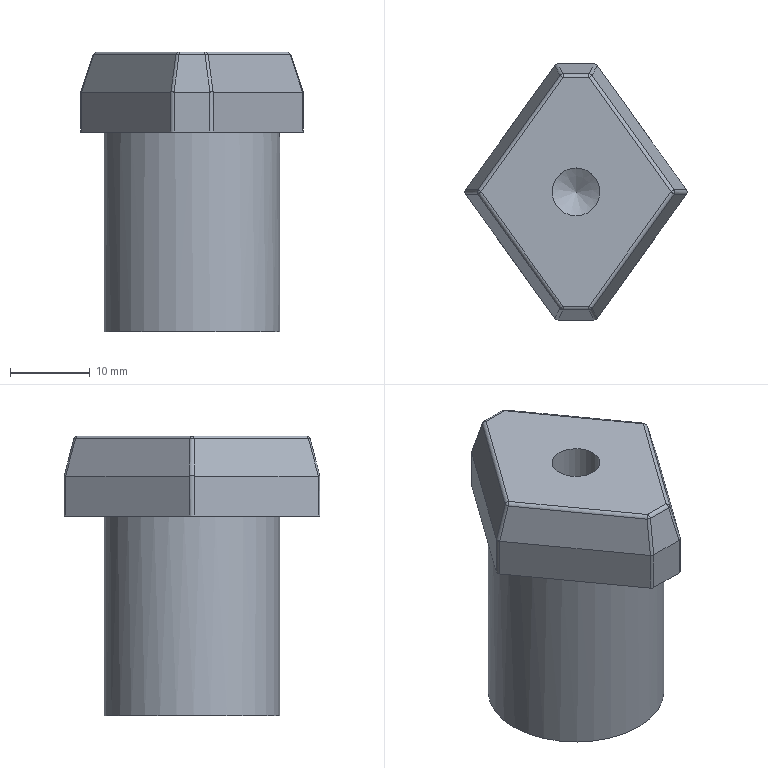Part | NX | features solid 2 | 1 solid | 45 faces | box 27.768 x 32 x 35 mm | volume 14194 mm3 | cylinder 20 | plane 18 | sphere 6 | cone 1 | commonest cylinder face diameters 1 x18 6 x1 22 x1
STEP:
#1=CARTESIAN_POINT('',(-816.022,-207.724,54.62));
#2=VERTEX_POINT('',#1);
#3=CARTESIAN_POINT('',(-816.022,-220.564,54.62));
#4=VERTEX_POINT('',#3);
#5=CARTESIAN_POINT('',(-807.09,-214.144,54.62));
#6=DIRECTION('',(0.,0.,1.));
#7=DIRECTION('',(1.,0.,0.));
#8=AXIS2_PLACEMENT_3D('',#5,#6,#7);
#9=CIRCLE('',#8,11.);
#10=EDGE_CURVE('',#2,#4,#9,.T.);
#11=ORIENTED_EDGE('',*,*,#10,.F.);
#12=CARTESIAN_POINT('',(-798.158,-207.724,54.62));
#13=VERTEX_POINT('',#12);
#14=CARTESIAN_POINT('',(-807.09,-214.144,54.62));
#15=DIRECTION('',(0.,0.,1.));
#16=DIRECTION('',(1.,0.,0.));
#17=AXIS2_PLACEMENT_3D('',#14,#15,#16);
#18=CIRCLE('',#17,11.);
#19=EDGE_CURVE('',#13,#2,#18,.T.);
#20=ORIENTED_EDGE('',*,*,#19,.F.);
#21=CARTESIAN_POINT('',(-798.158,-220.564,54.62));
#22=VERTEX_POINT('',#21);
#23=CARTESIAN_POINT('',(-807.09,-214.144,54.62));
#24=DIRECTION('',(0.,0.,1.));
#25=DIRECTION('',(1.,0.,0.));
#26=AXIS2_PLACEMENT_3D('',#23,#24,#25);
#27=CIRCLE('',#26,11.);
#28=EDGE_CURVE('',#22,#13,#27,.T.);
#29=ORIENTED_EDGE('',*,*,#28,.F.);
#30=CARTESIAN_POINT('',(-807.09,-214.144,54.62));
#31=DIRECTION('',(0.,0.,1.));
#32=DIRECTION('',(1.,0.,0.));
#33=AXIS2_PLACEMENT_3D('',#30,#31,#32);
#34=CIRCLE('',#33,11.);
#35=EDGE_CURVE('',#4,#22,#34,.T.);
#36=ORIENTED_EDGE('',*,*,#35,.F.);
#37=EDGE_LOOP('',(#11,#20,#29,#36));
#38=FACE_BOUND('',#37,.T.);
#39=CARTESIAN_POINT('',(-796.09,-214.144,29.62));
#40=VERTEX_POINT('',#39);
#41=CARTESIAN_POINT('',(-807.09,-214.144,29.62));
#42=DIRECTION('',(0.,0.,1.));
#43=DIRECTION('',(1.,0.,0.));
#44=AXIS2_PLACEMENT_3D('',#41,#42,#43);
#45=CIRCLE('',#44,11.);
#46=EDGE_CURVE('',#40,#40,#45,.T.);
#47=ORIENTED_EDGE('',*,*,#46,.T.);
#48=EDGE_LOOP('',(#47));
#49=FACE_BOUND('',#48,.T.);
#50=CARTESIAN_POINT('',(-807.09,-214.144,29.62));
#51=DIRECTION('',(0.,0.,1.));
#52=DIRECTION('',(0.,1.,0.));
#53=AXIS2_PLACEMENT_3D('',#50,#51,#52);
#54=CYLINDRICAL_SURFACE('',#53,11.);
#55=ADVANCED_FACE('',(#38,#49),#54,.T.);
#56=CARTESIAN_POINT('',(-820.88,-214.435,54.62));
#57=VERTEX_POINT('',#56);
#58=CARTESIAN_POINT('',(-816.321,-220.778,54.62));
#59=VERTEX_POINT('',#58);
#60=CARTESIAN_POINT('',(-821.09,-214.144,54.62));
#61=DIRECTION('',(0.5836,-0.812,0.));
#62=VECTOR('',#61,1000.);
#63=LINE('',#60,#62);
#64=EDGE_CURVE('',#57,#59,#63,.T.);
#65=ORIENTED_EDGE('',*,*,#64,.F.);
#66=CARTESIAN_POINT('',(-820.88,-213.852,54.62));
#67=VERTEX_POINT('',#66);
#68=CARTESIAN_POINT('',(-820.474,-214.144,54.62));
#69=DIRECTION('',(0.,0.,1.));
#70=DIRECTION('',(0.,1.,0.));
#71=AXIS2_PLACEMENT_3D('',#68,#69,#70);
#72=CIRCLE('',#71,0.5);
#73=EDGE_CURVE('',#57,#67,#72,.F.);
#74=ORIENTED_EDGE('',*,*,#73,.T.);
#75=CARTESIAN_POINT('',(-816.321,-207.509,54.62));
#76=VERTEX_POINT('',#75);
#77=CARTESIAN_POINT('',(-809.59,-198.144,54.62));
#78=DIRECTION('',(-0.5836,-0.812,0.));
#79=VECTOR('',#78,1000.);
#80=LINE('',#77,#79);
#81=EDGE_CURVE('',#76,#67,#80,.T.);
#82=ORIENTED_EDGE('',*,*,#81,.F.);
#83=CARTESIAN_POINT('',(-816.321,-207.509,54.62));
#84=CARTESIAN_POINT('',(-816.221,-207.58,54.62));
#85=CARTESIAN_POINT('',(-816.122,-207.652,54.62));
#86=CARTESIAN_POINT('',(-816.022,-207.724,54.62));
#87=B_SPLINE_CURVE_WITH_KNOTS('',3,(#83,#84,#85,#86),.UNSPECIFIED.,.F.,.F.,(4,4),(0.,0.2691),.UNSPECIFIED.);
#88=EDGE_CURVE('',#76,#2,#87,.T.);
#89=ORIENTED_EDGE('',*,*,#88,.T.);
#90=ORIENTED_EDGE('',*,*,#10,.T.);
#91=CARTESIAN_POINT('',(-816.022,-220.564,54.62));
#92=CARTESIAN_POINT('',(-816.122,-220.635,54.62));
#93=CARTESIAN_POINT('',(-816.221,-220.707,54.62));
#94=CARTESIAN_POINT('',(-816.321,-220.778,54.62));
#95=B_SPLINE_CURVE_WITH_KNOTS('',3,(#91,#92,#93,#94),.UNSPECIFIED.,.F.,.F.,(4,4),(0.7309,1.),.UNSPECIFIED.);
#96=EDGE_CURVE('',#59,#4,#95,.F.);
#97=ORIENTED_EDGE('',*,*,#96,.F.);
#98=EDGE_LOOP('',(#65,#74,#82,#89,#90,#97));
#99=FACE_BOUND('',#98,.T.);
#100=CARTESIAN_POINT('',(-804.59,-230.144,54.62));
#101=DIRECTION('',(0.,0.,1.));
#102=DIRECTION('',(0.,1.,0.));
#103=AXIS2_PLACEMENT_3D('',#100,#101,#102);
#104=PLANE('',#103);
#105=ADVANCED_FACE('',(#99),#104,.F.);
#106=CARTESIAN_POINT('',(-804.44,-229.935,54.62));
#107=VERTEX_POINT('',#106);
#108=CARTESIAN_POINT('',(-797.859,-220.778,54.62));
#109=VERTEX_POINT('',#108);
#110=CARTESIAN_POINT('',(-804.59,-230.144,54.62));
#111=DIRECTION('',(0.5836,0.812,0.));
#112=VECTOR('',#111,1000.);
#113=LINE('',#110,#112);
#114=EDGE_CURVE('',#107,#109,#113,.T.);
#115=ORIENTED_EDGE('',*,*,#114,.F.);
#116=CARTESIAN_POINT('',(-804.846,-230.144,54.62));
#117=VERTEX_POINT('',#116);
#118=CARTESIAN_POINT('',(-804.846,-229.644,54.62));
#119=DIRECTION('',(0.,0.,1.));
#120=DIRECTION('',(0.,1.,0.));
#121=AXIS2_PLACEMENT_3D('',#118,#119,#120);
#122=CIRCLE('',#121,0.5);
#123=EDGE_CURVE('',#107,#117,#122,.F.);
#124=ORIENTED_EDGE('',*,*,#123,.T.);
#125=CARTESIAN_POINT('',(-809.334,-230.144,54.62));
#126=VERTEX_POINT('',#125);
#127=CARTESIAN_POINT('',(-809.59,-230.144,54.62));
#128=DIRECTION('',(1.,0.,0.));
#129=VECTOR('',#128,1000.);
#130=LINE('',#127,#129);
#131=EDGE_CURVE('',#126,#117,#130,.T.);
#132=ORIENTED_EDGE('',*,*,#131,.F.);
#133=CARTESIAN_POINT('',(-809.74,-229.935,54.62));
#134=VERTEX_POINT('',#133);
#135=CARTESIAN_POINT('',(-809.334,-229.644,54.62));
#136=DIRECTION('',(0.,0.,1.));
#137=DIRECTION('',(0.,1.,0.));
#138=AXIS2_PLACEMENT_3D('',#135,#136,#137);
#139=CIRCLE('',#138,0.5);
#140=EDGE_CURVE('',#126,#134,#139,.F.);
#141=ORIENTED_EDGE('',*,*,#140,.T.);
#142=CARTESIAN_POINT('',(-821.09,-214.144,54.62));
#143=DIRECTION('',(0.5836,-0.812,0.));
#144=VECTOR('',#143,1000.);
#145=LINE('',#142,#144);
#146=EDGE_CURVE('',#59,#134,#145,.T.);
#147=ORIENTED_EDGE('',*,*,#146,.F.);
#148=ORIENTED_EDGE('',*,*,#96,.T.);
#149=ORIENTED_EDGE('',*,*,#35,.T.);
#150=CARTESIAN_POINT('',(-798.158,-220.564,54.62));
#151=CARTESIAN_POINT('',(-798.058,-220.635,54.62));
#152=CARTESIAN_POINT('',(-797.958,-220.707,54.62));
#153=CARTESIAN_POINT('',(-797.859,-220.778,54.62));
#154=B_SPLINE_CURVE_WITH_KNOTS('',3,(#150,#151,#152,#153),.UNSPECIFIED.,.F.,.F.,(4,4),(0.7309,1.),.UNSPECIFIED.);
#155=EDGE_CURVE('',#109,#22,#154,.F.);
#156=ORIENTED_EDGE('',*,*,#155,.F.);
#157=EDGE_LOOP('',(#115,#124,#132,#141,#147,#148,#149,#156));
#158=FACE_BOUND('',#157,.T.);
#159=CARTESIAN_POINT('',(-804.59,-230.144,54.62));
#160=DIRECTION('',(0.,0.,1.));
#161=DIRECTION('',(0.,1.,0.));
#162=AXIS2_PLACEMENT_3D('',#159,#160,#161);
#163=PLANE('',#162);
#164=ADVANCED_FACE('',(#158),#163,.F.);
#165=CARTESIAN_POINT('',(-793.3,-213.852,54.62));
#166=VERTEX_POINT('',#165);
#167=CARTESIAN_POINT('',(-797.859,-207.509,54.62));
#168=VERTEX_POINT('',#167);
#169=CARTESIAN_POINT('',(-793.09,-214.144,54.62));
#170=DIRECTION('',(-0.5836,0.812,0.));
#171=VECTOR('',#170,1000.);
#172=LINE('',#169,#171);
#173=EDGE_CURVE('',#166,#168,#172,.T.);
#174=ORIENTED_EDGE('',*,*,#173,.F.);
#175=CARTESIAN_POINT('',(-793.3,-214.435,54.62));
#176=VERTEX_POINT('',#175);
#177=CARTESIAN_POINT('',(-793.706,-214.144,54.62));
#178=DIRECTION('',(0.,0.,1.));
#179=DIRECTION('',(0.,1.,0.));
#180=AXIS2_PLACEMENT_3D('',#177,#178,#179);
#181=CIRCLE('',#180,0.5);
#182=EDGE_CURVE('',#166,#176,#181,.F.);
#183=ORIENTED_EDGE('',*,*,#182,.T.);
#184=CARTESIAN_POINT('',(-804.59,-230.144,54.62));
#185=DIRECTION('',(0.5836,0.812,0.));
#186=VECTOR('',#185,1000.);
#187=LINE('',#184,#186);
#188=EDGE_CURVE('',#109,#176,#187,.T.);
#189=ORIENTED_EDGE('',*,*,#188,.F.);
#190=ORIENTED_EDGE('',*,*,#155,.T.);
#191=ORIENTED_EDGE('',*,*,#28,.T.);
#192=CARTESIAN_POINT('',(-798.158,-207.724,54.62));
#193=CARTESIAN_POINT('',(-798.058,-207.652,54.62));
#194=CARTESIAN_POINT('',(-797.958,-207.58,54.62));
#195=CARTESIAN_POINT('',(-797.859,-207.509,54.62));
#196=B_SPLINE_CURVE_WITH_KNOTS('',3,(#192,#193,#194,#195),.UNSPECIFIED.,.F.,.F.,(4,4),(0.7309,1.),.UNSPECIFIED.);
#197=EDGE_CURVE('',#168,#13,#196,.F.);
#198=ORIENTED_EDGE('',*,*,#197,.F.);
#199=EDGE_LOOP('',(#174,#183,#189,#190,#191,#198));
#200=FACE_BOUND('',#199,.T.);
#201=CARTESIAN_POINT('',(-804.59,-230.144,54.62));
#202=DIRECTION('',(0.,0.,1.));
#203=DIRECTION('',(0.,1.,0.));
#204=AXIS2_PLACEMENT_3D('',#201,#202,#203);
#205=PLANE('',#204);
#206=ADVANCED_FACE('',(#200),#205,.F.);
#207=ORIENTED_EDGE('',*,*,#131,.T.);
#208=CARTESIAN_POINT('',(-804.846,-230.144,59.62));
#209=VERTEX_POINT('',#208);
#210=CARTESIAN_POINT('',(-804.846,-230.144,59.62));
#211=DIRECTION('',(0.,0.,-1.));
#212=VECTOR('',#211,1000.);
#213=LINE('',#210,#212);
#214=EDGE_CURVE('',#117,#209,#213,.F.);
#215=ORIENTED_EDGE('',*,*,#214,.T.);
#216=CARTESIAN_POINT('',(-809.334,-230.144,59.62));
#217=VERTEX_POINT('',#216);
#218=CARTESIAN_POINT('',(-809.59,-230.144,59.62));
#219=DIRECTION('',(1.,0.,0.));
#220=VECTOR('',#219,1000.);
#221=LINE('',#218,#220);
#222=EDGE_CURVE('',#217,#209,#221,.T.);
#223=ORIENTED_EDGE('',*,*,#222,.F.);
#224=CARTESIAN_POINT('',(-809.334,-230.144,59.62));
#225=DIRECTION('',(0.,0.,-1.));
#226=VECTOR('',#225,1000.);
#227=LINE('',#224,#226);
#228=EDGE_CURVE('',#217,#126,#227,.T.);
#229=ORIENTED_EDGE('',*,*,#228,.T.);
#230=EDGE_LOOP('',(#207,#215,#223,#229));
#231=FACE_BOUND('',#230,.T.);
#232=CARTESIAN_POINT('',(-809.59,-230.144,59.62));
#233=DIRECTION('',(0.,1.,0.));
#234=DIRECTION('',(0.,0.,-1.));
#235=AXIS2_PLACEMENT_3D('',#232,#233,#234);
#236=PLANE('',#235);
#237=ADVANCED_FACE('',(#231),#236,.F.);
#238=ORIENTED_EDGE('',*,*,#188,.T.);
#239=CARTESIAN_POINT('',(-793.3,-214.435,59.62));
#240=VERTEX_POINT('',#239);
#241=CARTESIAN_POINT('',(-793.3,-214.435,59.62));
#242=DIRECTION('',(0.,0.,-1.));
#243=VECTOR('',#242,1000.);
#244=LINE('',#241,#243);
#245=EDGE_CURVE('',#176,#240,#244,.F.);
#246=ORIENTED_EDGE('',*,*,#245,.T.);
#247=CARTESIAN_POINT('',(-804.44,-229.935,59.62));
#248=VERTEX_POINT('',#247);
#249=CARTESIAN_POINT('',(-804.59,-230.144,59.62));
#250=DIRECTION('',(0.5836,0.812,0.));
#251=VECTOR('',#250,1000.);
#252=LINE('',#249,#251);
#253=EDGE_CURVE('',#248,#240,#252,.T.);
#254=ORIENTED_EDGE('',*,*,#253,.F.);
#255=CARTESIAN_POINT('',(-804.44,-229.935,59.62));
#256=DIRECTION('',(0.,0.,-1.));
#257=VECTOR('',#256,1000.);
#258=LINE('',#255,#257);
#259=EDGE_CURVE('',#248,#107,#258,.T.);
#260=ORIENTED_EDGE('',*,*,#259,.T.);
#261=ORIENTED_EDGE('',*,*,#114,.T.);
#262=EDGE_LOOP('',(#238,#246,#254,#260,#261));
#263=FACE_BOUND('',#262,.T.);
#264=CARTESIAN_POINT('',(-804.59,-230.144,59.62));
#265=DIRECTION('',(-0.812,0.5836,0.));
#266=DIRECTION('',(-0.5836,-0.812,0.));
#267=AXIS2_PLACEMENT_3D('',#264,#265,#266);
#268=PLANE('',#267);
#269=ADVANCED_FACE('',(#263),#268,.F.);
#270=CARTESIAN_POINT('',(-804.44,-198.352,54.62));
#271=VERTEX_POINT('',#270);
#272=CARTESIAN_POINT('',(-793.09,-214.144,54.62));
#273=DIRECTION('',(-0.5836,0.812,0.));
#274=VECTOR('',#273,1000.);
#275=LINE('',#272,#274);
#276=EDGE_CURVE('',#168,#271,#275,.T.);
#277=ORIENTED_EDGE('',*,*,#276,.T.);
#278=CARTESIAN_POINT('',(-804.44,-198.352,59.62));
#279=VERTEX_POINT('',#278);
#280=CARTESIAN_POINT('',(-804.44,-198.352,59.62));
#281=DIRECTION('',(0.,0.,-1.));
#282=VECTOR('',#281,1000.);
#283=LINE('',#280,#282);
#284=EDGE_CURVE('',#271,#279,#283,.F.);
#285=ORIENTED_EDGE('',*,*,#284,.T.);
#286=CARTESIAN_POINT('',(-793.3,-213.852,59.62));
#287=VERTEX_POINT('',#286);
#288=CARTESIAN_POINT('',(-793.09,-214.144,59.62));
#289=DIRECTION('',(-0.5836,0.812,0.));
#290=VECTOR('',#289,1000.);
#291=LINE('',#288,#290);
#292=EDGE_CURVE('',#287,#279,#291,.T.);
#293=ORIENTED_EDGE('',*,*,#292,.F.);
#294=CARTESIAN_POINT('',(-793.3,-213.852,59.62));
#295=DIRECTION('',(0.,0.,-1.));
#296=VECTOR('',#295,1000.);
#297=LINE('',#294,#296);
#298=EDGE_CURVE('',#287,#166,#297,.T.);
#299=ORIENTED_EDGE('',*,*,#298,.T.);
#300=ORIENTED_EDGE('',*,*,#173,.T.);
#301=EDGE_LOOP('',(#277,#285,#293,#299,#300));
#302=FACE_BOUND('',#301,.T.);
#303=CARTESIAN_POINT('',(-793.09,-214.144,59.62));
#304=DIRECTION('',(-0.812,-0.5836,0.));
#305=DIRECTION('',(0.5836,-0.812,0.));
#306=AXIS2_PLACEMENT_3D('',#303,#304,#305);
#307=PLANE('',#306);
#308=ADVANCED_FACE('',(#302),#307,.F.);
#309=CARTESIAN_POINT('',(-804.846,-198.144,59.62));
#310=VERTEX_POINT('',#309);
#311=CARTESIAN_POINT('',(-809.334,-198.144,59.62));
#312=VERTEX_POINT('',#311);
#313=CARTESIAN_POINT('',(-804.59,-198.144,59.62));
#314=DIRECTION('',(-1.,0.,0.));
#315=VECTOR('',#314,1000.);
#316=LINE('',#313,#315);
#317=EDGE_CURVE('',#310,#312,#316,.T.);
#318=ORIENTED_EDGE('',*,*,#317,.F.);
#319=CARTESIAN_POINT('',(-804.846,-198.144,54.62));
#320=VERTEX_POINT('',#319);
#321=CARTESIAN_POINT('',(-804.846,-198.144,59.62));
#322=DIRECTION('',(0.,0.,-1.));
#323=VECTOR('',#322,1000.);
#324=LINE('',#321,#323);
#325=EDGE_CURVE('',#310,#320,#324,.T.);
#326=ORIENTED_EDGE('',*,*,#325,.T.);
#327=CARTESIAN_POINT('',(-809.334,-198.144,54.62));
#328=VERTEX_POINT('',#327);
#329=CARTESIAN_POINT('',(-804.59,-198.144,54.62));
#330=DIRECTION('',(-1.,0.,0.));
#331=VECTOR('',#330,1000.);
#332=LINE('',#329,#331);
#333=EDGE_CURVE('',#320,#328,#332,.T.);
#334=ORIENTED_EDGE('',*,*,#333,.T.);
#335=CARTESIAN_POINT('',(-809.334,-198.144,59.62));
#336=DIRECTION('',(0.,0.,-1.));
#337=VECTOR('',#336,1000.);
#338=LINE('',#335,#337);
#339=EDGE_CURVE('',#328,#312,#338,.F.);
#340=ORIENTED_EDGE('',*,*,#339,.T.);
#341=EDGE_LOOP('',(#318,#326,#334,#340));
#342=FACE_BOUND('',#341,.T.);
#343=CARTESIAN_POINT('',(-804.59,-198.144,59.62));
#344=DIRECTION('',(0.,-1.,0.));
#345=DIRECTION('',(0.,0.,1.));
#346=AXIS2_PLACEMENT_3D('',#343,#344,#345);
#347=PLANE('',#346);
#348=ADVANCED_FACE('',(#342),#347,.F.);
#349=ORIENTED_EDGE('',*,*,#81,.T.);
#350=CARTESIAN_POINT('',(-820.88,-213.852,59.62));
#351=VERTEX_POINT('',#350);
#352=CARTESIAN_POINT('',(-820.88,-213.852,59.62));
#353=DIRECTION('',(0.,0.,-1.));
#354=VECTOR('',#353,1000.);
#355=LINE('',#352,#354);
#356=EDGE_CURVE('',#67,#351,#355,.F.);
#357=ORIENTED_EDGE('',*,*,#356,.T.);
#358=CARTESIAN_POINT('',(-809.74,-198.352,59.62));
#359=VERTEX_POINT('',#358);
#360=CARTESIAN_POINT('',(-809.59,-198.144,59.62));
#361=DIRECTION('',(-0.5836,-0.812,0.));
#362=VECTOR('',#361,1000.);
#363=LINE('',#360,#362);
#364=EDGE_CURVE('',#359,#351,#363,.T.);
#365=ORIENTED_EDGE('',*,*,#364,.F.);
#366=CARTESIAN_POINT('',(-809.74,-198.352,54.62));
#367=VERTEX_POINT('',#366);
#368=CARTESIAN_POINT('',(-809.74,-198.352,59.62));
#369=DIRECTION('',(0.,0.,-1.));
#370=VECTOR('',#369,1000.);
#371=LINE('',#368,#370);
#372=EDGE_CURVE('',#359,#367,#371,.T.);
#373=ORIENTED_EDGE('',*,*,#372,.T.);
#374=CARTESIAN_POINT('',(-809.59,-198.144,54.62));
#375=DIRECTION('',(-0.5836,-0.812,0.));
#376=VECTOR('',#375,1000.);
#377=LINE('',#374,#376);
#378=EDGE_CURVE('',#367,#76,#377,.T.);
#379=ORIENTED_EDGE('',*,*,#378,.T.);
#380=EDGE_LOOP('',(#349,#357,#365,#373,#379));
#381=FACE_BOUND('',#380,.T.);
#382=CARTESIAN_POINT('',(-809.59,-198.144,59.62));
#383=DIRECTION('',(0.812,-0.5836,0.));
#384=DIRECTION('',(0.5836,0.812,0.));
#385=AXIS2_PLACEMENT_3D('',#382,#383,#384);
#386=PLANE('',#385);
#387=ADVANCED_FACE('',(#381),#386,.F.);
#388=ORIENTED_EDGE('',*,*,#146,.T.);
#389=CARTESIAN_POINT('',(-809.74,-229.935,59.62));
#390=VERTEX_POINT('',#389);
#391=CARTESIAN_POINT('',(-809.74,-229.935,59.62));
#392=DIRECTION('',(0.,0.,-1.));
#393=VECTOR('',#392,1000.);
#394=LINE('',#391,#393);
#395=EDGE_CURVE('',#134,#390,#394,.F.);
#396=ORIENTED_EDGE('',*,*,#395,.T.);
#397=CARTESIAN_POINT('',(-820.88,-214.435,59.62));
#398=VERTEX_POINT('',#397);
#399=CARTESIAN_POINT('',(-821.09,-214.144,59.62));
#400=DIRECTION('',(0.5836,-0.812,0.));
#401=VECTOR('',#400,1000.);
#402=LINE('',#399,#401);
#403=EDGE_CURVE('',#398,#390,#402,.T.);
#404=ORIENTED_EDGE('',*,*,#403,.F.);
#405=CARTESIAN_POINT('',(-820.88,-214.435,59.62));
#406=DIRECTION('',(0.,0.,-1.));
#407=VECTOR('',#406,1000.);
#408=LINE('',#405,#407);
#409=EDGE_CURVE('',#398,#57,#408,.T.);
#410=ORIENTED_EDGE('',*,*,#409,.T.);
#411=ORIENTED_EDGE('',*,*,#64,.T.);
#412=EDGE_LOOP('',(#388,#396,#404,#410,#411));
#413=FACE_BOUND('',#412,.T.);
#414=CARTESIAN_POINT('',(-821.09,-214.144,59.62));
#415=DIRECTION('',(0.812,0.5836,0.));
#416=DIRECTION('',(-0.5836,0.812,0.));
#417=AXIS2_PLACEMENT_3D('',#414,#415,#416);
#418=PLANE('',#417);
#419=ADVANCED_FACE('',(#413),#418,.F.);
#420=ORIENTED_EDGE('',*,*,#333,.F.);
#421=CARTESIAN_POINT('',(-804.846,-198.644,54.62));
#422=DIRECTION('',(0.,0.,1.));
#423=DIRECTION('',(0.,1.,0.));
#424=AXIS2_PLACEMENT_3D('',#421,#422,#423);
#425=CIRCLE('',#424,0.5);
#426=EDGE_CURVE('',#320,#271,#425,.F.);
#427=ORIENTED_EDGE('',*,*,#426,.T.);
#428=ORIENTED_EDGE('',*,*,#276,.F.);
#429=ORIENTED_EDGE('',*,*,#197,.T.);
#430=ORIENTED_EDGE('',*,*,#19,.T.);
#431=ORIENTED_EDGE('',*,*,#88,.F.);
#432=ORIENTED_EDGE('',*,*,#378,.F.);
#433=CARTESIAN_POINT('',(-809.334,-198.644,54.62));
#434=DIRECTION('',(0.,0.,1.));
#435=DIRECTION('',(0.,1.,0.));
#436=AXIS2_PLACEMENT_3D('',#433,#434,#435);
#437=CIRCLE('',#436,0.5);
#438=EDGE_CURVE('',#367,#328,#437,.F.);
#439=ORIENTED_EDGE('',*,*,#438,.T.);
#440=EDGE_LOOP('',(#420,#427,#428,#429,#430,#431,#432,#439));
#441=FACE_BOUND('',#440,.T.);
#442=CARTESIAN_POINT('',(-804.59,-230.144,54.62));
#443=DIRECTION('',(0.,0.,1.));
#444=DIRECTION('',(0.,1.,0.));
#445=AXIS2_PLACEMENT_3D('',#442,#443,#444);
#446=PLANE('',#445);
#447=ADVANCED_FACE('',(#441),#446,.F.);
#448=ORIENTED_EDGE('',*,*,#403,.T.);
#449=CARTESIAN_POINT('',(-809.734,-229.942,59.62));
#450=VERTEX_POINT('',#449);
#451=CARTESIAN_POINT('',(-809.334,-229.644,61.486));
#452=DIRECTION('',(-0.7843,-0.5637,0.2588));
#453=DIRECTION('',(-0.2102,-0.1511,-0.9659));
#454=AXIS2_PLACEMENT_3D('',#451,#452,#453);
#455=ELLIPSE('',#454,1.932,0.5);
#456=EDGE_CURVE('',#390,#450,#455,.T.);
#457=ORIENTED_EDGE('',*,*,#456,.T.);
#458=CARTESIAN_POINT('',(-809.098,-228.702,64.249));
#459=VERTEX_POINT('',#458);
#460=CARTESIAN_POINT('',(-809.539,-229.561,61.042));
#461=DIRECTION('',(0.1316,0.2566,0.9575));
#462=VECTOR('',#461,1000.);
#463=LINE('',#460,#462);
#464=EDGE_CURVE('',#450,#459,#463,.T.);
#465=ORIENTED_EDGE('',*,*,#464,.T.);
#466=CARTESIAN_POINT('',(-819.36,-214.425,64.249));
#467=VERTEX_POINT('',#466);
#468=CARTESIAN_POINT('',(-819.521,-214.201,64.249));
#469=DIRECTION('',(0.5836,-0.812,0.));
#470=VECTOR('',#469,1000.);
#471=LINE('',#468,#470);
#472=EDGE_CURVE('',#459,#467,#471,.F.);
#473=ORIENTED_EDGE('',*,*,#472,.T.);
#474=CARTESIAN_POINT('',(-820.887,-214.425,59.621));
#475=VERTEX_POINT('',#474);
#476=CARTESIAN_POINT('',(-820.439,-214.425,60.979));
#477=DIRECTION('',(0.3134,0.,0.9496));
#478=VECTOR('',#477,1000.);
#479=LINE('',#476,#478);
#480=EDGE_CURVE('',#467,#475,#479,.F.);
#481=ORIENTED_EDGE('',*,*,#480,.T.);
#482=CARTESIAN_POINT('',(-820.474,-214.144,61.486));
#483=DIRECTION('',(-0.7843,-0.5637,0.2588));
#484=DIRECTION('',(-0.2102,-0.1511,-0.9659));
#485=AXIS2_PLACEMENT_3D('',#482,#483,#484);
#486=ELLIPSE('',#485,1.932,0.5);
#487=EDGE_CURVE('',#475,#398,#486,.T.);
#488=ORIENTED_EDGE('',*,*,#487,.T.);
#489=EDGE_LOOP('',(#448,#457,#465,#473,#481,#488));
#490=FACE_BOUND('',#489,.T.);
#491=CARTESIAN_POINT('',(-816.321,-220.778,59.62));
#492=DIRECTION('',(-0.7843,-0.5637,0.2588));
#493=DIRECTION('',(0.5836,-0.812,0.));
#494=AXIS2_PLACEMENT_3D('',#491,#492,#493);
#495=PLANE('',#494);
#496=ADVANCED_FACE('',(#490),#495,.T.);
#497=ORIENTED_EDGE('',*,*,#222,.T.);
#498=CARTESIAN_POINT('',(-804.838,-230.143,59.62));
#499=VERTEX_POINT('',#498);
#500=CARTESIAN_POINT('',(-804.846,-229.644,61.486));
#501=DIRECTION('',(0.,-0.9659,0.2588));
#502=DIRECTION('',(0.,-0.2588,-0.9659));
#503=AXIS2_PLACEMENT_3D('',#500,#501,#502);
#504=ELLIPSE('',#503,1.932,0.5);
#505=EDGE_CURVE('',#209,#499,#504,.T.);
#506=ORIENTED_EDGE('',*,*,#505,.T.);
#507=CARTESIAN_POINT('',(-805.474,-228.903,64.249));
#508=VERTEX_POINT('',#507);
#509=CARTESIAN_POINT('',(-804.877,-230.067,59.904));
#510=DIRECTION('',(-0.1316,0.2566,0.9575));
#511=VECTOR('',#510,1000.);
#512=LINE('',#509,#511);
#513=EDGE_CURVE('',#499,#508,#512,.T.);
#514=ORIENTED_EDGE('',*,*,#513,.T.);
#515=CARTESIAN_POINT('',(-808.706,-228.903,64.249));
#516=VERTEX_POINT('',#515);
#517=CARTESIAN_POINT('',(-808.903,-228.903,64.249));
#518=DIRECTION('',(1.,0.,0.));
#519=VECTOR('',#518,1000.);
#520=LINE('',#517,#519);
#521=EDGE_CURVE('',#508,#516,#520,.F.);
#522=ORIENTED_EDGE('',*,*,#521,.T.);
#523=CARTESIAN_POINT('',(-809.342,-230.143,59.62));
#524=VERTEX_POINT('',#523);
#525=CARTESIAN_POINT('',(-809.303,-230.067,59.904));
#526=DIRECTION('',(0.1316,0.2566,0.9575));
#527=VECTOR('',#526,1000.);
#528=LINE('',#525,#527);
#529=EDGE_CURVE('',#516,#524,#528,.F.);
#530=ORIENTED_EDGE('',*,*,#529,.T.);
#531=CARTESIAN_POINT('',(-809.334,-229.644,61.486));
#532=DIRECTION('',(0.,-0.9659,0.2588));
#533=DIRECTION('',(0.,-0.2588,-0.9659));
#534=AXIS2_PLACEMENT_3D('',#531,#532,#533);
#535=ELLIPSE('',#534,1.932,0.5);
#536=EDGE_CURVE('',#524,#217,#535,.T.);
#537=ORIENTED_EDGE('',*,*,#536,.T.);
#538=EDGE_LOOP('',(#497,#506,#514,#522,#530,#537));
#539=FACE_BOUND('',#538,.T.);
#540=CARTESIAN_POINT('',(-807.09,-230.144,59.62));
#541=DIRECTION('',(0.,-0.9659,0.2588));
#542=DIRECTION('',(0.,0.2588,0.9659));
#543=AXIS2_PLACEMENT_3D('',#540,#541,#542);
#544=PLANE('',#543);
#545=ADVANCED_FACE('',(#539),#544,.T.);
#546=ORIENTED_EDGE('',*,*,#253,.T.);
#547=CARTESIAN_POINT('',(-793.293,-214.425,59.621));
#548=VERTEX_POINT('',#547);
#549=CARTESIAN_POINT('',(-793.706,-214.144,61.486));
#550=DIRECTION('',(0.7843,-0.5637,0.2588));
#551=DIRECTION('',(0.2102,-0.1511,-0.9659));
#552=AXIS2_PLACEMENT_3D('',#549,#550,#551);
#553=ELLIPSE('',#552,1.932,0.5);
#554=EDGE_CURVE('',#240,#548,#553,.T.);
#555=ORIENTED_EDGE('',*,*,#554,.T.);
#556=CARTESIAN_POINT('',(-794.82,-214.425,64.249));
#557=VERTEX_POINT('',#556);
#558=CARTESIAN_POINT('',(-793.741,-214.425,60.979));
#559=DIRECTION('',(-0.3134,0.,0.9496));
#560=VECTOR('',#559,1000.);
#561=LINE('',#558,#560);
#562=EDGE_CURVE('',#548,#557,#561,.T.);
#563=ORIENTED_EDGE('',*,*,#562,.T.);
#564=CARTESIAN_POINT('',(-805.081,-228.702,64.249));
#565=VERTEX_POINT('',#564);
#566=CARTESIAN_POINT('',(-805.196,-228.862,64.249));
#567=DIRECTION('',(0.5836,0.812,0.));
#568=VECTOR('',#567,1000.);
#569=LINE('',#566,#568);
#570=EDGE_CURVE('',#557,#565,#569,.F.);
#571=ORIENTED_EDGE('',*,*,#570,.T.);
#572=CARTESIAN_POINT('',(-804.445,-229.942,59.62));
#573=VERTEX_POINT('',#572);
#574=CARTESIAN_POINT('',(-804.641,-229.561,61.042));
#575=DIRECTION('',(-0.1316,0.2566,0.9575));
#576=VECTOR('',#575,1000.);
#577=LINE('',#574,#576);
#578=EDGE_CURVE('',#565,#573,#577,.F.);
#579=ORIENTED_EDGE('',*,*,#578,.T.);
#580=CARTESIAN_POINT('',(-804.846,-229.644,61.486));
#581=DIRECTION('',(0.7843,-0.5637,0.2588));
#582=DIRECTION('',(0.2102,-0.1511,-0.9659));
#583=AXIS2_PLACEMENT_3D('',#580,#581,#582);
#584=ELLIPSE('',#583,1.932,0.5);
#585=EDGE_CURVE('',#573,#248,#584,.T.);
#586=ORIENTED_EDGE('',*,*,#585,.T.);
#587=EDGE_LOOP('',(#546,#555,#563,#571,#579,#586));
#588=FACE_BOUND('',#587,.T.);
#589=CARTESIAN_POINT('',(-797.859,-220.778,59.62));
#590=DIRECTION('',(0.7843,-0.5637,0.2588));
#591=DIRECTION('',(0.5836,0.812,0.));
#592=AXIS2_PLACEMENT_3D('',#589,#590,#591);
#593=PLANE('',#592);
#594=ADVANCED_FACE('',(#588),#593,.T.);
#595=ORIENTED_EDGE('',*,*,#292,.T.);
#596=CARTESIAN_POINT('',(-804.445,-198.345,59.62));
#597=VERTEX_POINT('',#596);
#598=CARTESIAN_POINT('',(-804.846,-198.644,61.486));
#599=DIRECTION('',(0.7843,0.5637,0.2588));
#600=DIRECTION('',(0.2102,0.1511,-0.9659));
#601=AXIS2_PLACEMENT_3D('',#598,#599,#600);
#602=ELLIPSE('',#601,1.932,0.5);
#603=EDGE_CURVE('',#279,#597,#602,.T.);
#604=ORIENTED_EDGE('',*,*,#603,.T.);
#605=CARTESIAN_POINT('',(-805.081,-199.585,64.249));
#606=VERTEX_POINT('',#605);
#607=CARTESIAN_POINT('',(-804.641,-198.726,61.042));
#608=DIRECTION('',(-0.1316,-0.2566,0.9575));
#609=VECTOR('',#608,1000.);
#610=LINE('',#607,#609);
#611=EDGE_CURVE('',#597,#606,#610,.T.);
#612=ORIENTED_EDGE('',*,*,#611,.T.);
#613=CARTESIAN_POINT('',(-794.82,-213.862,64.249));
#614=VERTEX_POINT('',#613);
#615=CARTESIAN_POINT('',(-794.659,-214.086,64.249));
#616=DIRECTION('',(-0.5836,0.812,0.));
#617=VECTOR('',#616,1000.);
#618=LINE('',#615,#617);
#619=EDGE_CURVE('',#606,#614,#618,.F.);
#620=ORIENTED_EDGE('',*,*,#619,.T.);
#621=CARTESIAN_POINT('',(-793.293,-213.862,59.621));
#622=VERTEX_POINT('',#621);
#623=CARTESIAN_POINT('',(-793.741,-213.862,60.979));
#624=DIRECTION('',(-0.3134,0.,0.9496));
#625=VECTOR('',#624,1000.);
#626=LINE('',#623,#625);
#627=EDGE_CURVE('',#614,#622,#626,.F.);
#628=ORIENTED_EDGE('',*,*,#627,.T.);
#629=CARTESIAN_POINT('',(-793.706,-214.144,61.486));
#630=DIRECTION('',(0.7843,0.5637,0.2588));
#631=DIRECTION('',(0.2102,0.1511,-0.9659));
#632=AXIS2_PLACEMENT_3D('',#629,#630,#631);
#633=ELLIPSE('',#632,1.932,0.5);
#634=EDGE_CURVE('',#622,#287,#633,.T.);
#635=ORIENTED_EDGE('',*,*,#634,.T.);
#636=EDGE_LOOP('',(#595,#604,#612,#620,#628,#635));
#637=FACE_BOUND('',#636,.T.);
#638=CARTESIAN_POINT('',(-797.859,-207.509,59.62));
#639=DIRECTION('',(0.7843,0.5637,0.2588));
#640=DIRECTION('',(-0.5836,0.812,0.));
#641=AXIS2_PLACEMENT_3D('',#638,#639,#640);
#642=PLANE('',#641);
#643=ADVANCED_FACE('',(#637),#642,.T.);
#644=CARTESIAN_POINT('',(-805.474,-199.384,64.249));
#645=VERTEX_POINT('',#644);
#646=CARTESIAN_POINT('',(-804.838,-198.144,59.62));
#647=VERTEX_POINT('',#646);
#648=CARTESIAN_POINT('',(-804.877,-198.22,59.904));
#649=DIRECTION('',(-0.1316,-0.2566,0.9575));
#650=VECTOR('',#649,1000.);
#651=LINE('',#648,#650);
#652=EDGE_CURVE('',#645,#647,#651,.F.);
#653=ORIENTED_EDGE('',*,*,#652,.T.);
#654=CARTESIAN_POINT('',(-804.846,-198.644,61.486));
#655=DIRECTION('',(0.,0.9659,0.2588));
#656=DIRECTION('',(0.,0.2588,-0.9659));
#657=AXIS2_PLACEMENT_3D('',#654,#655,#656);
#658=ELLIPSE('',#657,1.932,0.5);
#659=EDGE_CURVE('',#647,#310,#658,.T.);
#660=ORIENTED_EDGE('',*,*,#659,.T.);
#661=ORIENTED_EDGE('',*,*,#317,.T.);
#662=CARTESIAN_POINT('',(-809.342,-198.144,59.62));
#663=VERTEX_POINT('',#662);
#664=CARTESIAN_POINT('',(-809.334,-198.644,61.486));
#665=DIRECTION('',(0.,0.9659,0.2588));
#666=DIRECTION('',(0.,0.2588,-0.9659));
#667=AXIS2_PLACEMENT_3D('',#664,#665,#666);
#668=ELLIPSE('',#667,1.932,0.5);
#669=EDGE_CURVE('',#312,#663,#668,.T.);
#670=ORIENTED_EDGE('',*,*,#669,.T.);
#671=CARTESIAN_POINT('',(-808.706,-199.384,64.249));
#672=VERTEX_POINT('',#671);
#673=CARTESIAN_POINT('',(-809.303,-198.22,59.904));
#674=DIRECTION('',(0.1316,-0.2566,0.9575));
#675=VECTOR('',#674,1000.);
#676=LINE('',#673,#675);
#677=EDGE_CURVE('',#663,#672,#676,.T.);
#678=ORIENTED_EDGE('',*,*,#677,.T.);
#679=CARTESIAN_POINT('',(-805.277,-199.384,64.249));
#680=DIRECTION('',(-1.,0.,0.));
#681=VECTOR('',#680,1000.);
#682=LINE('',#679,#681);
#683=EDGE_CURVE('',#672,#645,#682,.F.);
#684=ORIENTED_EDGE('',*,*,#683,.T.);
#685=EDGE_LOOP('',(#653,#660,#661,#670,#678,#684));
#686=FACE_BOUND('',#685,.T.);
#687=CARTESIAN_POINT('',(-807.09,-198.144,59.62));
#688=DIRECTION('',(0.,0.9659,0.2588));
#689=DIRECTION('',(0.,0.2588,-0.9659));
#690=AXIS2_PLACEMENT_3D('',#687,#688,#689);
#691=PLANE('',#690);
#692=ADVANCED_FACE('',(#686),#691,.T.);
#693=ORIENTED_EDGE('',*,*,#364,.T.);
#694=CARTESIAN_POINT('',(-820.887,-213.862,59.621));
#695=VERTEX_POINT('',#694);
#696=CARTESIAN_POINT('',(-820.474,-214.144,61.486));
#697=DIRECTION('',(-0.7843,0.5637,0.2588));
#698=DIRECTION('',(-0.2102,0.1511,-0.9659));
#699=AXIS2_PLACEMENT_3D('',#696,#697,#698);
#700=ELLIPSE('',#699,1.932,0.5);
#701=EDGE_CURVE('',#351,#695,#700,.T.);
#702=ORIENTED_EDGE('',*,*,#701,.T.);
#703=CARTESIAN_POINT('',(-819.36,-213.862,64.249));
#704=VERTEX_POINT('',#703);
#705=CARTESIAN_POINT('',(-820.439,-213.862,60.979));
#706=DIRECTION('',(0.3134,0.,0.9496));
#707=VECTOR('',#706,1000.);
#708=LINE('',#705,#707);
#709=EDGE_CURVE('',#695,#704,#708,.T.);
#710=ORIENTED_EDGE('',*,*,#709,.T.);
#711=CARTESIAN_POINT('',(-809.098,-199.585,64.249));
#712=VERTEX_POINT('',#711);
#713=CARTESIAN_POINT('',(-808.984,-199.425,64.249));
#714=DIRECTION('',(-0.5836,-0.812,0.));
#715=VECTOR('',#714,1000.);
#716=LINE('',#713,#715);
#717=EDGE_CURVE('',#704,#712,#716,.F.);
#718=ORIENTED_EDGE('',*,*,#717,.T.);
#719=CARTESIAN_POINT('',(-809.734,-198.345,59.62));
#720=VERTEX_POINT('',#719);
#721=CARTESIAN_POINT('',(-809.539,-198.726,61.042));
#722=DIRECTION('',(0.1316,-0.2566,0.9575));
#723=VECTOR('',#722,1000.);
#724=LINE('',#721,#723);
#725=EDGE_CURVE('',#712,#720,#724,.F.);
#726=ORIENTED_EDGE('',*,*,#725,.T.);
#727=CARTESIAN_POINT('',(-809.334,-198.644,61.486));
#728=DIRECTION('',(-0.7843,0.5637,0.2588));
#729=DIRECTION('',(-0.2102,0.1511,-0.9659));
#730=AXIS2_PLACEMENT_3D('',#727,#728,#729);
#731=ELLIPSE('',#730,1.932,0.5);
#732=EDGE_CURVE('',#720,#359,#731,.T.);
#733=ORIENTED_EDGE('',*,*,#732,.T.);
#734=EDGE_LOOP('',(#693,#702,#710,#718,#726,#733));
#735=FACE_BOUND('',#734,.T.);
#736=CARTESIAN_POINT('',(-816.321,-207.509,59.62));
#737=DIRECTION('',(-0.7843,0.5637,0.2588));
#738=DIRECTION('',(-0.5836,-0.812,0.));
#739=AXIS2_PLACEMENT_3D('',#736,#737,#738);
#740=PLANE('',#739);
#741=ADVANCED_FACE('',(#735),#740,.T.);
#742=CARTESIAN_POINT('',(-805.474,-228.42,64.62));
#743=VERTEX_POINT('',#742);
#744=CARTESIAN_POINT('',(-795.212,-214.144,64.62));
#745=VERTEX_POINT('',#744);
#746=CARTESIAN_POINT('',(-795.051,-213.92,64.62));
#747=DIRECTION('',(-0.5836,-0.812,0.));
#748=VECTOR('',#747,1000.);
#749=LINE('',#746,#748);
#750=EDGE_CURVE('',#743,#745,#749,.F.);
#751=ORIENTED_EDGE('',*,*,#750,.T.);
#752=CARTESIAN_POINT('',(-805.474,-199.867,64.62));
#753=VERTEX_POINT('',#752);
#754=CARTESIAN_POINT('',(-805.588,-199.707,64.62));
#755=DIRECTION('',(0.5836,-0.812,0.));
#756=VECTOR('',#755,1000.);
#757=LINE('',#754,#756);
#758=EDGE_CURVE('',#745,#753,#757,.F.);
#759=ORIENTED_EDGE('',*,*,#758,.T.);
#760=CARTESIAN_POINT('',(-808.706,-199.867,64.62));
#761=VERTEX_POINT('',#760);
#762=CARTESIAN_POINT('',(-808.903,-199.867,64.62));
#763=DIRECTION('',(1.,0.,0.));
#764=VECTOR('',#763,1000.);
#765=LINE('',#762,#764);
#766=EDGE_CURVE('',#753,#761,#765,.F.);
#767=ORIENTED_EDGE('',*,*,#766,.T.);
#768=CARTESIAN_POINT('',(-818.968,-214.144,64.62));
#769=VERTEX_POINT('',#768);
#770=CARTESIAN_POINT('',(-819.128,-214.367,64.62));
#771=DIRECTION('',(0.5836,0.812,0.));
#772=VECTOR('',#771,1000.);
#773=LINE('',#770,#772);
#774=EDGE_CURVE('',#761,#769,#773,.F.);
#775=ORIENTED_EDGE('',*,*,#774,.T.);
#776=CARTESIAN_POINT('',(-808.706,-228.42,64.62));
#777=VERTEX_POINT('',#776);
#778=CARTESIAN_POINT('',(-808.591,-228.58,64.62));
#779=DIRECTION('',(-0.5836,0.812,0.));
#780=VECTOR('',#779,1000.);
#781=LINE('',#778,#780);
#782=EDGE_CURVE('',#769,#777,#781,.F.);
#783=ORIENTED_EDGE('',*,*,#782,.T.);
#784=CARTESIAN_POINT('',(-805.277,-228.42,64.62));
#785=DIRECTION('',(-1.,0.,0.));
#786=VECTOR('',#785,1000.);
#787=LINE('',#784,#786);
#788=EDGE_CURVE('',#777,#743,#787,.F.);
#789=ORIENTED_EDGE('',*,*,#788,.T.);
#790=EDGE_LOOP('',(#751,#759,#767,#775,#783,#789));
#791=FACE_BOUND('',#790,.T.);
#792=CARTESIAN_POINT('',(-807.09,-217.144,64.62));
#793=VERTEX_POINT('',#792);
#794=CARTESIAN_POINT('',(-807.09,-214.144,64.62));
#795=DIRECTION('',(0.,0.,-1.));
#796=DIRECTION('',(0.,-1.,0.));
#797=AXIS2_PLACEMENT_3D('',#794,#795,#796);
#798=CIRCLE('',#797,3.);
#799=EDGE_CURVE('',#793,#793,#798,.T.);
#800=ORIENTED_EDGE('',*,*,#799,.T.);
#801=EDGE_LOOP('',(#800));
#802=FACE_BOUND('',#801,.T.);
#803=CARTESIAN_POINT('',(-807.09,-233.622,64.62));
#804=DIRECTION('',(0.,0.,1.));
#805=DIRECTION('',(0.,1.,0.));
#806=AXIS2_PLACEMENT_3D('',#803,#804,#805);
#807=PLANE('',#806);
#808=ADVANCED_FACE('',(#791,#802),#807,.T.);
#809=ORIENTED_EDGE('',*,*,#46,.F.);
#810=EDGE_LOOP('',(#809));
#811=FACE_BOUND('',#810,.T.);
#812=CARTESIAN_POINT('',(-807.09,-214.144,29.62));
#813=DIRECTION('',(0.,0.,1.));
#814=DIRECTION('',(0.,1.,0.));
#815=AXIS2_PLACEMENT_3D('',#812,#813,#814);
#816=PLANE('',#815);
#817=ADVANCED_FACE('',(#811),#816,.F.);
#818=CARTESIAN_POINT('',(-807.09,-217.144,54.62));
#819=VERTEX_POINT('',#818);
#820=CARTESIAN_POINT('',(-807.09,-214.144,54.62));
#821=DIRECTION('',(0.,0.,-1.));
#822=DIRECTION('',(0.,-1.,0.));
#823=AXIS2_PLACEMENT_3D('',#820,#821,#822);
#824=CIRCLE('',#823,3.);
#825=EDGE_CURVE('',#819,#819,#824,.T.);
#826=ORIENTED_EDGE('',*,*,#825,.F.);
#827=EDGE_LOOP('',(#826));
#828=FACE_BOUND('',#827,.T.);
#829=CARTESIAN_POINT('',(-807.09,-214.144,52.817));
#830=VERTEX_POINT('',#829);
#831=VERTEX_LOOP('',#830);
#832=FACE_BOUND('',#831,.T.);
#833=CARTESIAN_POINT('',(-807.09,-214.144,54.62));
#834=DIRECTION('',(0.,0.,1.));
#835=DIRECTION('',(0.,1.,0.));
#836=AXIS2_PLACEMENT_3D('',#833,#834,#835);
#837=CONICAL_SURFACE('',#836,3.,1.03);
#838=ADVANCED_FACE('',(#828,#832),#837,.F.);
#839=ORIENTED_EDGE('',*,*,#825,.T.);
#840=EDGE_LOOP('',(#839));
#841=FACE_BOUND('',#840,.T.);
#842=ORIENTED_EDGE('',*,*,#799,.F.);
#843=EDGE_LOOP('',(#842));
#844=FACE_BOUND('',#843,.T.);
#845=CARTESIAN_POINT('',(-807.09,-214.144,64.62));
#846=DIRECTION('',(0.,0.,-1.));
#847=DIRECTION('',(0.,-1.,0.));
#848=AXIS2_PLACEMENT_3D('',#845,#846,#847);
#849=CYLINDRICAL_SURFACE('',#848,3.);
#850=ADVANCED_FACE('',(#841,#844),#849,.F.);
#851=ORIENTED_EDGE('',*,*,#228,.F.);
#852=ORIENTED_EDGE('',*,*,#536,.F.);
#853=CARTESIAN_POINT('',(-809.334,-229.644,59.554));
#854=DIRECTION('',(-0.06649,-0.1297,-0.9893));
#855=DIRECTION('',(-0.4514,-0.8803,0.1457));
#856=AXIS2_PLACEMENT_3D('',#853,#854,#855);
#857=ELLIPSE('',#856,0.5054,0.5);
#858=EDGE_CURVE('',#450,#524,#857,.F.);
#859=ORIENTED_EDGE('',*,*,#858,.F.);
#860=ORIENTED_EDGE('',*,*,#456,.F.);
#861=ORIENTED_EDGE('',*,*,#395,.F.);
#862=ORIENTED_EDGE('',*,*,#140,.F.);
#863=EDGE_LOOP('',(#851,#852,#859,#860,#861,#862));
#864=FACE_BOUND('',#863,.T.);
#865=CARTESIAN_POINT('',(-809.334,-229.644,59.62));
#866=DIRECTION('',(0.,0.,-1.));
#867=DIRECTION('',(0.,-1.,0.));
#868=AXIS2_PLACEMENT_3D('',#865,#866,#867);
#869=CYLINDRICAL_SURFACE('',#868,0.5);
#870=ADVANCED_FACE('',(#864),#869,.T.);
#871=ORIENTED_EDGE('',*,*,#858,.T.);
#872=ORIENTED_EDGE('',*,*,#529,.F.);
#873=CARTESIAN_POINT('',(-808.706,-228.42,64.12));
#874=DIRECTION('',(0.1316,0.2566,0.9575));
#875=DIRECTION('',(0.,0.9659,-0.2588));
#876=AXIS2_PLACEMENT_3D('',#873,#874,#875);
#877=CIRCLE('',#876,0.5);
#878=EDGE_CURVE('',#459,#516,#877,.T.);
#879=ORIENTED_EDGE('',*,*,#878,.F.);
#880=ORIENTED_EDGE('',*,*,#464,.F.);
#881=EDGE_LOOP('',(#871,#872,#879,#880));
#882=FACE_BOUND('',#881,.T.);
#883=CARTESIAN_POINT('',(-809.303,-229.585,59.774));
#884=DIRECTION('',(-0.1316,-0.2566,-0.9575));
#885=DIRECTION('',(0.,-0.9659,0.2588));
#886=AXIS2_PLACEMENT_3D('',#883,#884,#885);
#887=CYLINDRICAL_SURFACE('',#886,0.5);
#888=ADVANCED_FACE('',(#882),#887,.T.);
#889=ORIENTED_EDGE('',*,*,#259,.F.);
#890=ORIENTED_EDGE('',*,*,#585,.F.);
#891=CARTESIAN_POINT('',(-804.846,-229.644,59.554));
#892=DIRECTION('',(0.06649,-0.1297,-0.9893));
#893=DIRECTION('',(0.4514,-0.8803,0.1457));
#894=AXIS2_PLACEMENT_3D('',#891,#892,#893);
#895=ELLIPSE('',#894,0.5054,0.5);
#896=EDGE_CURVE('',#499,#573,#895,.F.);
#897=ORIENTED_EDGE('',*,*,#896,.F.);
#898=ORIENTED_EDGE('',*,*,#505,.F.);
#899=ORIENTED_EDGE('',*,*,#214,.F.);
#900=ORIENTED_EDGE('',*,*,#123,.F.);
#901=EDGE_LOOP('',(#889,#890,#897,#898,#899,#900));
#902=FACE_BOUND('',#901,.T.);
#903=CARTESIAN_POINT('',(-804.846,-229.644,59.62));
#904=DIRECTION('',(0.,0.,-1.));
#905=DIRECTION('',(0.,-1.,0.));
#906=AXIS2_PLACEMENT_3D('',#903,#904,#905);
#907=CYLINDRICAL_SURFACE('',#906,0.5);
#908=ADVANCED_FACE('',(#902),#907,.T.);
#909=CARTESIAN_POINT('',(-808.706,-228.42,64.12));
#910=DIRECTION('',(0.5836,-0.812,0.));
#911=DIRECTION('',(0.812,0.5836,0.));
#912=AXIS2_PLACEMENT_3D('',#909,#910,#911);
#913=CIRCLE('',#912,0.5);
#914=EDGE_CURVE('',#459,#777,#913,.F.);
#915=ORIENTED_EDGE('',*,*,#914,.F.);
#916=ORIENTED_EDGE('',*,*,#878,.T.);
#917=CARTESIAN_POINT('',(-808.706,-228.42,64.12));
#918=DIRECTION('',(-1.,0.,0.));
#919=DIRECTION('',(0.,0.,1.));
#920=AXIS2_PLACEMENT_3D('',#917,#918,#919);
#921=CIRCLE('',#920,0.5);
#922=EDGE_CURVE('',#777,#516,#921,.F.);
#923=ORIENTED_EDGE('',*,*,#922,.F.);
#924=EDGE_LOOP('',(#915,#916,#923));
#925=FACE_BOUND('',#924,.T.);
#926=CARTESIAN_POINT('',(-808.706,-228.42,64.12));
#927=DIRECTION('',(0.,0.,1.));
#928=DIRECTION('',(0.,1.,0.));
#929=AXIS2_PLACEMENT_3D('',#926,#927,#928);
#930=SPHERICAL_SURFACE('',#929,0.5);
#931=ADVANCED_FACE('',(#925),#930,.T.);
#932=ORIENTED_EDGE('',*,*,#409,.F.);
#933=ORIENTED_EDGE('',*,*,#487,.F.);
#934=CARTESIAN_POINT('',(-820.474,-214.144,59.554));
#935=DIRECTION('',(-0.1587,0.,-0.9873));
#936=DIRECTION('',(-0.9873,0.,0.1587));
#937=AXIS2_PLACEMENT_3D('',#934,#935,#936);
#938=ELLIPSE('',#937,0.5064,0.5);
#939=EDGE_CURVE('',#695,#475,#938,.F.);
#940=ORIENTED_EDGE('',*,*,#939,.F.);
#941=ORIENTED_EDGE('',*,*,#701,.F.);
#942=ORIENTED_EDGE('',*,*,#356,.F.);
#943=ORIENTED_EDGE('',*,*,#73,.F.);
#944=EDGE_LOOP('',(#932,#933,#940,#941,#942,#943));
#945=FACE_BOUND('',#944,.T.);
#946=CARTESIAN_POINT('',(-820.474,-214.144,59.62));
#947=DIRECTION('',(0.,0.,-1.));
#948=DIRECTION('',(0.,-1.,0.));
#949=AXIS2_PLACEMENT_3D('',#946,#947,#948);
#950=CYLINDRICAL_SURFACE('',#949,0.5);
#951=ADVANCED_FACE('',(#945),#950,.T.);
#952=ORIENTED_EDGE('',*,*,#896,.T.);
#953=ORIENTED_EDGE('',*,*,#578,.F.);
#954=CARTESIAN_POINT('',(-805.474,-228.42,64.12));
#955=DIRECTION('',(-0.1316,0.2566,0.9575));
#956=DIRECTION('',(0.,0.9659,-0.2588));
#957=AXIS2_PLACEMENT_3D('',#954,#955,#956);
#958=CIRCLE('',#957,0.5);
#959=EDGE_CURVE('',#508,#565,#958,.T.);
#960=ORIENTED_EDGE('',*,*,#959,.F.);
#961=ORIENTED_EDGE('',*,*,#513,.F.);
#962=EDGE_LOOP('',(#952,#953,#960,#961));
#963=FACE_BOUND('',#962,.T.);
#964=CARTESIAN_POINT('',(-805.033,-229.28,60.912));
#965=DIRECTION('',(0.1316,-0.2566,-0.9575));
#966=DIRECTION('',(0.,-0.9659,0.2588));
#967=AXIS2_PLACEMENT_3D('',#964,#965,#966);
#968=CYLINDRICAL_SURFACE('',#967,0.5);
#969=ADVANCED_FACE('',(#963),#968,.T.);
#970=ORIENTED_EDGE('',*,*,#922,.T.);
#971=ORIENTED_EDGE('',*,*,#521,.F.);
#972=CARTESIAN_POINT('',(-805.474,-228.42,64.12));
#973=DIRECTION('',(1.,0.,0.));
#974=DIRECTION('',(0.,1.,0.));
#975=AXIS2_PLACEMENT_3D('',#972,#973,#974);
#976=CIRCLE('',#975,0.5);
#977=EDGE_CURVE('',#743,#508,#976,.T.);
#978=ORIENTED_EDGE('',*,*,#977,.F.);
#979=ORIENTED_EDGE('',*,*,#788,.F.);
#980=EDGE_LOOP('',(#970,#971,#978,#979));
#981=FACE_BOUND('',#980,.T.);
#982=CARTESIAN_POINT('',(-807.09,-228.42,64.12));
#983=DIRECTION('',(1.,0.,0.));
#984=DIRECTION('',(0.,0.,-1.));
#985=AXIS2_PLACEMENT_3D('',#982,#983,#984);
#986=CYLINDRICAL_SURFACE('',#985,0.5);
#987=ADVANCED_FACE('',(#981),#986,.T.);
#988=ORIENTED_EDGE('',*,*,#914,.T.);
#989=ORIENTED_EDGE('',*,*,#782,.F.);
#990=CARTESIAN_POINT('',(-818.968,-214.144,64.12));
#991=DIRECTION('',(-0.5836,0.812,0.));
#992=DIRECTION('',(-0.812,-0.5836,0.));
#993=AXIS2_PLACEMENT_3D('',#990,#991,#992);
#994=CIRCLE('',#993,0.5);
#995=EDGE_CURVE('',#467,#769,#994,.T.);
#996=ORIENTED_EDGE('',*,*,#995,.F.);
#997=ORIENTED_EDGE('',*,*,#472,.F.);
#998=EDGE_LOOP('',(#988,#989,#996,#997));
#999=FACE_BOUND('',#998,.T.);
#1000=CARTESIAN_POINT('',(-805.69,-232.616,64.12));
#1001=DIRECTION('',(0.5836,-0.812,0.));
#1002=DIRECTION('',(0.812,0.5836,0.));
#1003=AXIS2_PLACEMENT_3D('',#1000,#1001,#1002);
#1004=CYLINDRICAL_SURFACE('',#1003,0.5);
#1005=ADVANCED_FACE('',(#999),#1004,.T.);
#1006=ORIENTED_EDGE('',*,*,#939,.T.);
#1007=ORIENTED_EDGE('',*,*,#480,.F.);
#1008=CARTESIAN_POINT('',(-818.968,-214.144,64.12));
#1009=DIRECTION('',(0.3134,0.,0.9496));
#1010=DIRECTION('',(0.9496,0.,-0.3134));
#1011=AXIS2_PLACEMENT_3D('',#1008,#1009,#1010);
#1012=CIRCLE('',#1011,0.5);
#1013=EDGE_CURVE('',#704,#467,#1012,.T.);
#1014=ORIENTED_EDGE('',*,*,#1013,.F.);
#1015=ORIENTED_EDGE('',*,*,#709,.F.);
#1016=EDGE_LOOP('',(#1006,#1007,#1014,#1015));
#1017=FACE_BOUND('',#1016,.T.);
#1018=CARTESIAN_POINT('',(-820.047,-214.144,60.849));
#1019=DIRECTION('',(-0.3134,0.,-0.9496));
#1020=DIRECTION('',(-0.9496,0.,0.3134));
#1021=AXIS2_PLACEMENT_3D('',#1018,#1019,#1020);
#1022=CYLINDRICAL_SURFACE('',#1021,0.5);
#1023=ADVANCED_FACE('',(#1017),#1022,.T.);
#1024=ORIENTED_EDGE('',*,*,#298,.F.);
#1025=ORIENTED_EDGE('',*,*,#634,.F.);
#1026=CARTESIAN_POINT('',(-793.706,-214.144,59.554));
#1027=DIRECTION('',(0.1587,0.,-0.9873));
#1028=DIRECTION('',(0.9873,0.,0.1587));
#1029=AXIS2_PLACEMENT_3D('',#1026,#1027,#1028);
#1030=ELLIPSE('',#1029,0.5064,0.5);
#1031=EDGE_CURVE('',#548,#622,#1030,.F.);
#1032=ORIENTED_EDGE('',*,*,#1031,.F.);
#1033=ORIENTED_EDGE('',*,*,#554,.F.);
#1034=ORIENTED_EDGE('',*,*,#245,.F.);
#1035=ORIENTED_EDGE('',*,*,#182,.F.);
#1036=EDGE_LOOP('',(#1024,#1025,#1032,#1033,#1034,#1035));
#1037=FACE_BOUND('',#1036,.T.);
#1038=CARTESIAN_POINT('',(-793.706,-214.144,59.62));
#1039=DIRECTION('',(0.,0.,-1.));
#1040=DIRECTION('',(0.,-1.,0.));
#1041=AXIS2_PLACEMENT_3D('',#1038,#1039,#1040);
#1042=CYLINDRICAL_SURFACE('',#1041,0.5);
#1043=ADVANCED_FACE('',(#1037),#1042,.T.);
#1044=ORIENTED_EDGE('',*,*,#977,.T.);
#1045=ORIENTED_EDGE('',*,*,#959,.T.);
#1046=CARTESIAN_POINT('',(-805.474,-228.42,64.12));
#1047=DIRECTION('',(-0.5836,-0.812,0.));
#1048=DIRECTION('',(0.812,-0.5836,0.));
#1049=AXIS2_PLACEMENT_3D('',#1046,#1047,#1048);
#1050=CIRCLE('',#1049,0.5);
#1051=EDGE_CURVE('',#743,#565,#1050,.F.);
#1052=ORIENTED_EDGE('',*,*,#1051,.F.);
#1053=EDGE_LOOP('',(#1044,#1045,#1052));
#1054=FACE_BOUND('',#1053,.T.);
#1055=CARTESIAN_POINT('',(-805.474,-228.42,64.12));
#1056=DIRECTION('',(0.,0.,1.));
#1057=DIRECTION('',(0.,1.,0.));
#1058=AXIS2_PLACEMENT_3D('',#1055,#1056,#1057);
#1059=SPHERICAL_SURFACE('',#1058,0.5);
#1060=ADVANCED_FACE('',(#1054),#1059,.T.);
#1061=ORIENTED_EDGE('',*,*,#1013,.T.);
#1062=ORIENTED_EDGE('',*,*,#995,.T.);
#1063=CARTESIAN_POINT('',(-818.968,-214.144,64.12));
#1064=DIRECTION('',(-0.5836,-0.812,0.));
#1065=DIRECTION('',(0.812,-0.5836,0.));
#1066=AXIS2_PLACEMENT_3D('',#1063,#1064,#1065);
#1067=CIRCLE('',#1066,0.5);
#1068=EDGE_CURVE('',#704,#769,#1067,.F.);
#1069=ORIENTED_EDGE('',*,*,#1068,.F.);
#1070=EDGE_LOOP('',(#1061,#1062,#1069));
#1071=FACE_BOUND('',#1070,.T.);
#1072=CARTESIAN_POINT('',(-818.968,-214.144,64.12));
#1073=DIRECTION('',(0.,0.,1.));
#1074=DIRECTION('',(0.,1.,0.));
#1075=AXIS2_PLACEMENT_3D('',#1072,#1073,#1074);
#1076=SPHERICAL_SURFACE('',#1075,0.5);
#1077=ADVANCED_FACE('',(#1071),#1076,.T.);
#1078=ORIENTED_EDGE('',*,*,#372,.F.);
#1079=ORIENTED_EDGE('',*,*,#732,.F.);
#1080=CARTESIAN_POINT('',(-809.334,-198.644,59.554));
#1081=DIRECTION('',(-0.06649,0.1297,-0.9893));
#1082=DIRECTION('',(-0.4514,0.8803,0.1457));
#1083=AXIS2_PLACEMENT_3D('',#1080,#1081,#1082);
#1084=ELLIPSE('',#1083,0.5054,0.5);
#1085=EDGE_CURVE('',#663,#720,#1084,.F.);
#1086=ORIENTED_EDGE('',*,*,#1085,.F.);
#1087=ORIENTED_EDGE('',*,*,#669,.F.);
#1088=ORIENTED_EDGE('',*,*,#339,.F.);
#1089=ORIENTED_EDGE('',*,*,#438,.F.);
#1090=EDGE_LOOP('',(#1078,#1079,#1086,#1087,#1088,#1089));
#1091=FACE_BOUND('',#1090,.T.);
#1092=CARTESIAN_POINT('',(-809.334,-198.644,59.62));
#1093=DIRECTION('',(0.,0.,-1.));
#1094=DIRECTION('',(0.,-1.,0.));
#1095=AXIS2_PLACEMENT_3D('',#1092,#1093,#1094);
#1096=CYLINDRICAL_SURFACE('',#1095,0.5);
#1097=ADVANCED_FACE('',(#1091),#1096,.T.);
#1098=ORIENTED_EDGE('',*,*,#1031,.T.);
#1099=ORIENTED_EDGE('',*,*,#627,.F.);
#1100=CARTESIAN_POINT('',(-795.212,-214.144,64.12));
#1101=DIRECTION('',(-0.3134,0.,0.9496));
#1102=DIRECTION('',(0.9496,0.,0.3134));
#1103=AXIS2_PLACEMENT_3D('',#1100,#1101,#1102);
#1104=CIRCLE('',#1103,0.5);
#1105=EDGE_CURVE('',#557,#614,#1104,.T.);
#1106=ORIENTED_EDGE('',*,*,#1105,.F.);
#1107=ORIENTED_EDGE('',*,*,#562,.F.);
#1108=EDGE_LOOP('',(#1098,#1099,#1106,#1107));
#1109=FACE_BOUND('',#1108,.T.);
#1110=CARTESIAN_POINT('',(-794.133,-214.144,60.849));
#1111=DIRECTION('',(0.3134,0.,-0.9496));
#1112=DIRECTION('',(-0.9496,0.,-0.3134));
#1113=AXIS2_PLACEMENT_3D('',#1110,#1111,#1112);
#1114=CYLINDRICAL_SURFACE('',#1113,0.5);
#1115=ADVANCED_FACE('',(#1109),#1114,.T.);
#1116=ORIENTED_EDGE('',*,*,#1051,.T.);
#1117=ORIENTED_EDGE('',*,*,#570,.F.);
#1118=CARTESIAN_POINT('',(-795.212,-214.144,64.12));
#1119=DIRECTION('',(0.5836,0.812,0.));
#1120=DIRECTION('',(-0.812,0.5836,0.));
#1121=AXIS2_PLACEMENT_3D('',#1118,#1119,#1120);
#1122=CIRCLE('',#1121,0.5);
#1123=EDGE_CURVE('',#745,#557,#1122,.T.);
#1124=ORIENTED_EDGE('',*,*,#1123,.F.);
#1125=ORIENTED_EDGE('',*,*,#750,.F.);
#1126=EDGE_LOOP('',(#1116,#1117,#1124,#1125));
#1127=FACE_BOUND('',#1126,.T.);
#1128=CARTESIAN_POINT('',(-808.489,-232.616,64.12));
#1129=DIRECTION('',(0.5836,0.812,0.));
#1130=DIRECTION('',(-0.812,0.5836,0.));
#1131=AXIS2_PLACEMENT_3D('',#1128,#1129,#1130);
#1132=CYLINDRICAL_SURFACE('',#1131,0.5);
#1133=ADVANCED_FACE('',(#1127),#1132,.T.);
#1134=ORIENTED_EDGE('',*,*,#1068,.T.);
#1135=ORIENTED_EDGE('',*,*,#774,.F.);
#1136=CARTESIAN_POINT('',(-808.706,-199.867,64.12));
#1137=DIRECTION('',(0.5836,0.812,0.));
#1138=DIRECTION('',(-0.812,0.5836,0.));
#1139=AXIS2_PLACEMENT_3D('',#1136,#1137,#1138);
#1140=CIRCLE('',#1139,0.5);
#1141=EDGE_CURVE('',#712,#761,#1140,.T.);
#1142=ORIENTED_EDGE('',*,*,#1141,.F.);
#1143=ORIENTED_EDGE('',*,*,#717,.F.);
#1144=EDGE_LOOP('',(#1134,#1135,#1142,#1143));
#1145=FACE_BOUND('',#1144,.T.);
#1146=CARTESIAN_POINT('',(-824.153,-221.358,64.12));
#1147=DIRECTION('',(-0.5836,-0.812,0.));
#1148=DIRECTION('',(0.812,-0.5836,0.));
#1149=AXIS2_PLACEMENT_3D('',#1146,#1147,#1148);
#1150=CYLINDRICAL_SURFACE('',#1149,0.5);
#1151=ADVANCED_FACE('',(#1145),#1150,.T.);
#1152=ORIENTED_EDGE('',*,*,#1085,.T.);
#1153=ORIENTED_EDGE('',*,*,#725,.F.);
#1154=CARTESIAN_POINT('',(-808.706,-199.867,64.12));
#1155=DIRECTION('',(0.1316,-0.2566,0.9575));
#1156=DIRECTION('',(0.,0.9659,0.2588));
#1157=AXIS2_PLACEMENT_3D('',#1154,#1155,#1156);
#1158=CIRCLE('',#1157,0.5);
#1159=EDGE_CURVE('',#672,#712,#1158,.T.);
#1160=ORIENTED_EDGE('',*,*,#1159,.F.);
#1161=ORIENTED_EDGE('',*,*,#677,.F.);
#1162=EDGE_LOOP('',(#1152,#1153,#1160,#1161));
#1163=FACE_BOUND('',#1162,.T.);
#1164=CARTESIAN_POINT('',(-809.147,-199.007,60.912));
#1165=DIRECTION('',(-0.1316,0.2566,-0.9575));
#1166=DIRECTION('',(0.,-0.9659,-0.2588));
#1167=AXIS2_PLACEMENT_3D('',#1164,#1165,#1166);
#1168=CYLINDRICAL_SURFACE('',#1167,0.5);
#1169=ADVANCED_FACE('',(#1163),#1168,.T.);
#1170=ORIENTED_EDGE('',*,*,#1123,.T.);
#1171=ORIENTED_EDGE('',*,*,#1105,.T.);
#1172=CARTESIAN_POINT('',(-795.212,-214.144,64.12));
#1173=DIRECTION('',(0.5836,-0.812,0.));
#1174=DIRECTION('',(0.812,0.5836,0.));
#1175=AXIS2_PLACEMENT_3D('',#1172,#1173,#1174);
#1176=CIRCLE('',#1175,0.5);
#1177=EDGE_CURVE('',#745,#614,#1176,.F.);
#1178=ORIENTED_EDGE('',*,*,#1177,.F.);
#1179=EDGE_LOOP('',(#1170,#1171,#1178));
#1180=FACE_BOUND('',#1179,.T.);
#1181=CARTESIAN_POINT('',(-795.212,-214.144,64.12));
#1182=DIRECTION('',(0.,0.,1.));
#1183=DIRECTION('',(0.,1.,0.));
#1184=AXIS2_PLACEMENT_3D('',#1181,#1182,#1183);
#1185=SPHERICAL_SURFACE('',#1184,0.5);
#1186=ADVANCED_FACE('',(#1180),#1185,.T.);
#1187=ORIENTED_EDGE('',*,*,#1159,.T.);
#1188=ORIENTED_EDGE('',*,*,#1141,.T.);
#1189=CARTESIAN_POINT('',(-808.706,-199.867,64.12));
#1190=DIRECTION('',(-1.,0.,0.));
#1191=DIRECTION('',(0.,-1.,0.));
#1192=AXIS2_PLACEMENT_3D('',#1189,#1190,#1191);
#1193=CIRCLE('',#1192,0.5);
#1194=EDGE_CURVE('',#672,#761,#1193,.F.);
#1195=ORIENTED_EDGE('',*,*,#1194,.F.);
#1196=EDGE_LOOP('',(#1187,#1188,#1195));
#1197=FACE_BOUND('',#1196,.T.);
#1198=CARTESIAN_POINT('',(-808.706,-199.867,64.12));
#1199=DIRECTION('',(0.,0.,1.));
#1200=DIRECTION('',(0.,1.,0.));
#1201=AXIS2_PLACEMENT_3D('',#1198,#1199,#1200);
#1202=SPHERICAL_SURFACE('',#1201,0.5);
#1203=ADVANCED_FACE('',(#1197),#1202,.T.);
#1204=ORIENTED_EDGE('',*,*,#1177,.T.);
#1205=ORIENTED_EDGE('',*,*,#619,.F.);
#1206=CARTESIAN_POINT('',(-805.474,-199.867,64.12));
#1207=DIRECTION('',(-0.5836,0.812,0.));
#1208=DIRECTION('',(-0.812,-0.5836,0.));
#1209=AXIS2_PLACEMENT_3D('',#1206,#1207,#1208);
#1210=CIRCLE('',#1209,0.5);
#1211=EDGE_CURVE('',#753,#606,#1210,.T.);
#1212=ORIENTED_EDGE('',*,*,#1211,.F.);
#1213=ORIENTED_EDGE('',*,*,#758,.F.);
#1214=EDGE_LOOP('',(#1204,#1205,#1212,#1213));
#1215=FACE_BOUND('',#1214,.T.);
#1216=CARTESIAN_POINT('',(-790.027,-221.358,64.12));
#1217=DIRECTION('',(-0.5836,0.812,0.));
#1218=DIRECTION('',(-0.812,-0.5836,0.));
#1219=AXIS2_PLACEMENT_3D('',#1216,#1217,#1218);
#1220=CYLINDRICAL_SURFACE('',#1219,0.5);
#1221=ADVANCED_FACE('',(#1215),#1220,.T.);
#1222=ORIENTED_EDGE('',*,*,#1194,.T.);
#1223=ORIENTED_EDGE('',*,*,#766,.F.);
#1224=CARTESIAN_POINT('',(-805.474,-199.867,64.12));
#1225=DIRECTION('',(1.,0.,0.));
#1226=DIRECTION('',(0.,0.,-1.));
#1227=AXIS2_PLACEMENT_3D('',#1224,#1225,#1226);
#1228=CIRCLE('',#1227,0.5);
#1229=EDGE_CURVE('',#645,#753,#1228,.T.);
#1230=ORIENTED_EDGE('',*,*,#1229,.F.);
#1231=ORIENTED_EDGE('',*,*,#683,.F.);
#1232=EDGE_LOOP('',(#1222,#1223,#1230,#1231));
#1233=FACE_BOUND('',#1232,.T.);
#1234=CARTESIAN_POINT('',(-807.09,-199.867,64.12));
#1235=DIRECTION('',(-1.,0.,0.));
#1236=DIRECTION('',(0.,0.,1.));
#1237=AXIS2_PLACEMENT_3D('',#1234,#1235,#1236);
#1238=CYLINDRICAL_SURFACE('',#1237,0.5);
#1239=ADVANCED_FACE('',(#1233),#1238,.T.);
#1240=ORIENTED_EDGE('',*,*,#1229,.T.);
#1241=ORIENTED_EDGE('',*,*,#1211,.T.);
#1242=CARTESIAN_POINT('',(-805.474,-199.867,64.12));
#1243=DIRECTION('',(-0.1316,-0.2566,0.9575));
#1244=DIRECTION('',(0.,0.9659,0.2588));
#1245=AXIS2_PLACEMENT_3D('',#1242,#1243,#1244);
#1246=CIRCLE('',#1245,0.5);
#1247=EDGE_CURVE('',#645,#606,#1246,.F.);
#1248=ORIENTED_EDGE('',*,*,#1247,.F.);
#1249=EDGE_LOOP('',(#1240,#1241,#1248));
#1250=FACE_BOUND('',#1249,.T.);
#1251=CARTESIAN_POINT('',(-805.474,-199.867,64.12));
#1252=DIRECTION('',(0.,0.,1.));
#1253=DIRECTION('',(0.,1.,0.));
#1254=AXIS2_PLACEMENT_3D('',#1251,#1252,#1253);
#1255=SPHERICAL_SURFACE('',#1254,0.5);
#1256=ADVANCED_FACE('',(#1250),#1255,.T.);
#1257=ORIENTED_EDGE('',*,*,#1247,.T.);
#1258=ORIENTED_EDGE('',*,*,#611,.F.);
#1259=CARTESIAN_POINT('',(-804.846,-198.644,59.554));
#1260=DIRECTION('',(0.06649,0.1297,-0.9893));
#1261=DIRECTION('',(0.4514,0.8803,0.1457));
#1262=AXIS2_PLACEMENT_3D('',#1259,#1260,#1261);
#1263=ELLIPSE('',#1262,0.5054,0.5);
#1264=EDGE_CURVE('',#647,#597,#1263,.T.);
#1265=ORIENTED_EDGE('',*,*,#1264,.F.);
#1266=ORIENTED_EDGE('',*,*,#652,.F.);
#1267=EDGE_LOOP('',(#1257,#1258,#1265,#1266));
#1268=FACE_BOUND('',#1267,.T.);
#1269=CARTESIAN_POINT('',(-804.877,-198.702,59.774));
#1270=DIRECTION('',(0.1316,0.2566,-0.9575));
#1271=DIRECTION('',(0.,-0.9659,-0.2588));
#1272=AXIS2_PLACEMENT_3D('',#1269,#1270,#1271);
#1273=CYLINDRICAL_SURFACE('',#1272,0.5);
#1274=ADVANCED_FACE('',(#1268),#1273,.T.);
#1275=ORIENTED_EDGE('',*,*,#603,.F.);
#1276=ORIENTED_EDGE('',*,*,#284,.F.);
#1277=ORIENTED_EDGE('',*,*,#426,.F.);
#1278=ORIENTED_EDGE('',*,*,#325,.F.);
#1279=ORIENTED_EDGE('',*,*,#659,.F.);
#1280=ORIENTED_EDGE('',*,*,#1264,.T.);
#1281=EDGE_LOOP('',(#1275,#1276,#1277,#1278,#1279,#1280));
#1282=FACE_BOUND('',#1281,.T.);
#1283=CARTESIAN_POINT('',(-804.846,-198.644,59.62));
#1284=DIRECTION('',(0.,0.,-1.));
#1285=DIRECTION('',(0.,-1.,0.));
#1286=AXIS2_PLACEMENT_3D('',#1283,#1284,#1285);
#1287=CYLINDRICAL_SURFACE('',#1286,0.5);
#1288=ADVANCED_FACE('',(#1282),#1287,.T.);
#1289=CLOSED_SHELL('',(#55,#105,#164,#206,#237,#269,#308,#348,#387,#419,#447,#496,#545,#594,#643,#692,#741,#808,#817,#838,#850,#870,#888,#908,#931,#951,#969,#987,#1005,#1023,#1043,#1060,#1077,#1097,#1115,#1133,#1151,#1169,#1186,#1203,#1221,#1239,#1256,#1274,#1288));
#1290=MANIFOLD_SOLID_BREP('',#1289);
#1291=(LENGTH_UNIT()NAMED_UNIT(*)SI_UNIT(.MILLI.,.METRE.));
#1292=UNCERTAINTY_MEASURE_WITH_UNIT(LENGTH_MEASURE(0.0508),#1291,'','');
#1293=(NAMED_UNIT(*)PLANE_ANGLE_UNIT()SI_UNIT($,.RADIAN.));
#1294=(NAMED_UNIT(*)SI_UNIT($,.STERADIAN.)SOLID_ANGLE_UNIT());
#1295=(GEOMETRIC_REPRESENTATION_CONTEXT(3)GLOBAL_UNCERTAINTY_ASSIGNED_CONTEXT((#1292))GLOBAL_UNIT_ASSIGNED_CONTEXT((#1291,#1293,#1294))REPRESENTATION_CONTEXT('',''));
#1296=ADVANCED_BREP_SHAPE_REPRESENTATION('',(#1290),#1295);